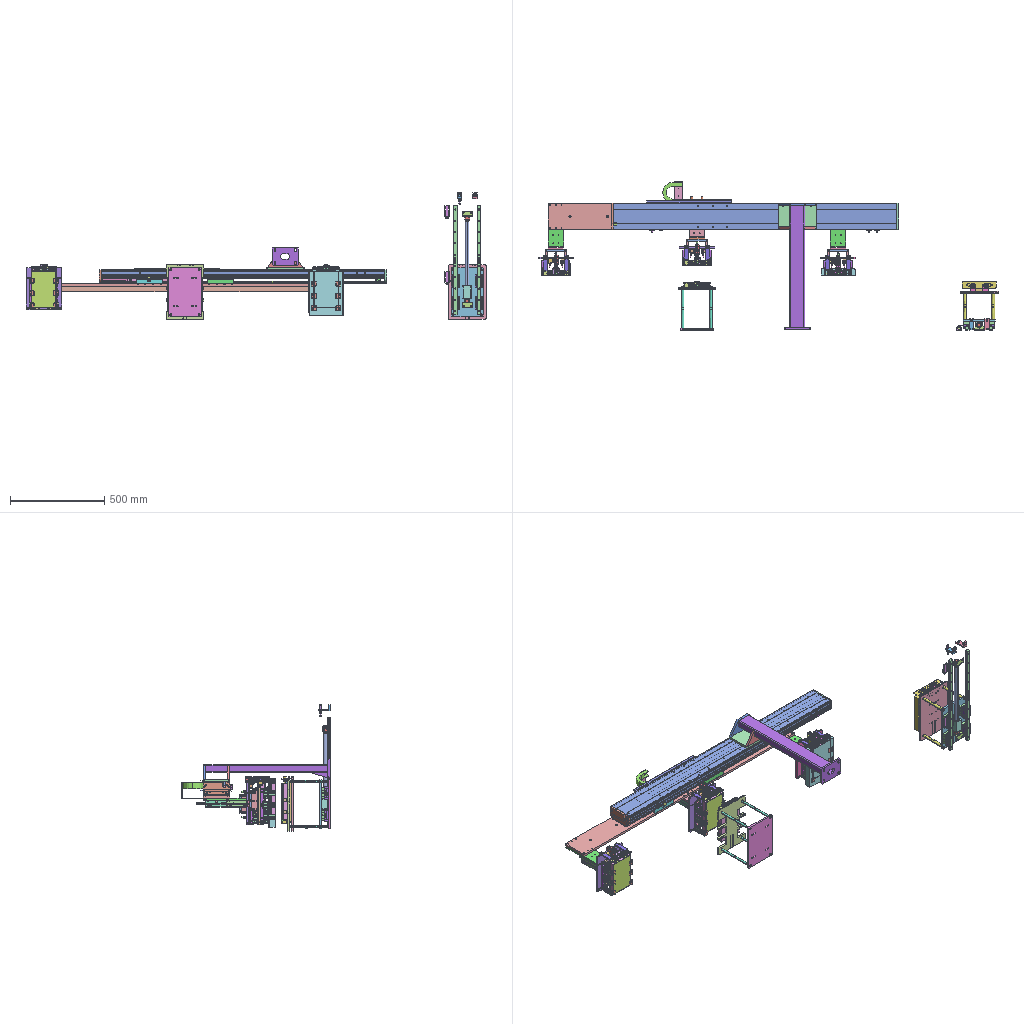Assembly | STEP file | 111 different items | 296 placed | box 2445 x 787 x 674 mm
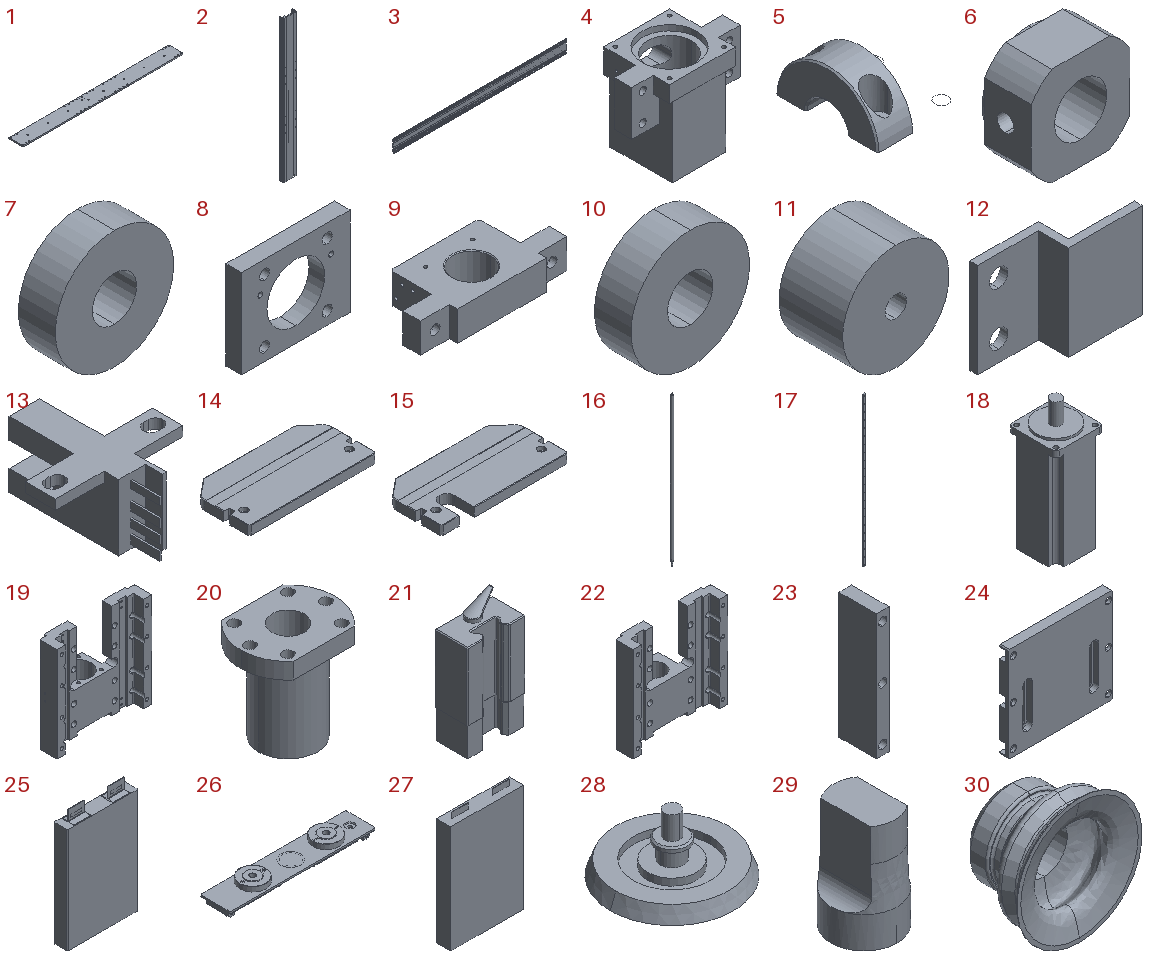Parts list (item | name | quantity | parent item | size | volume):
1 | 0-19-01 Sliding plate | x1 | in 33 | 1583 x 140 x 12 mm | 2630174 mm3
2 | SM140A-20-1140D-140A-600 Base SF600 | x1 | in SM140A-20-1140D-E | 140 x 48 x 1508 mm | 3406004 mm3
3 | SM140A-20-1140D-140A-600 Upper cover SF600 | x1 | in SM140A-20-1140D-E | 1524 x 10 x 112 mm | 391118 mm3
4 | SM140A-20-1140D-140A-600 Front bearing seat | x1 | in SM140A-20-1140D-E | 99 x 60 x 82 mm | 158063 mm3
5 | SM140A-20-1140D-140A-600 Coupling | x1 | in SM140A-20-1140D-E | - | -
6 | SM140A-20-1140D-140A-600 Lock nut | x1 | in SM140A-20-1140D-E | 19 x 10 x 19 mm | 2441 mm3
7 | SM140A-20-1140D-140A-600 Front bearing | x2 | in SM140A-20-1140D-E | 32 x 10 x 32 mm | 6912 mm3
8 | SM140A-20-1140D-140A-600 Pressure plate | x1 | in SM140A-20-1140D-E | 49 x 7 x 40 mm | 8955 mm3
9 | SM140A-20-1140D-140A-600 Rear bearing seat | x1 | in SM140A-20-1140D-E | 99 x 45.5 x 20 mm | 51169 mm3
10 | SM140A-20-1140D-140A-600 Rear end bearing | x1 | in SM140A-20-1140D-E | 26 x 8 x 26 mm | 3619 mm3
11 | SM140A-20-1140D-140A-600 Buffer pad | x4 | in SM140A-20-1140D-E | 15 x 9 x 15 mm | 1428 mm3
12 | SM140A-20-1140D-140A-600 External sensor plate | x1 | in SM140A-20-1140D-E | 25.5 x 7.25 x 18 mm | 814.887 mm3
13 | SM140A-20-1140D-140A-600ABSR | x3 | in SM140A-20-1140D-E | 26 x 28.4 x 13.5 mm | 1855 mm3
14 | SM140A-20-1140D-140A-600 Rear end plate | x1 | in SM140A-20-1140D-E | 140 x 70.5 x 10 mm | 88188 mm3
15 | SM140A-20-1140D-140A-600 Front end plate | x1 | in SM140A-20-1140D-E | 140 x 70.5 x 10 mm | 83515 mm3
16 | SM140A-20-1140D-140A-60016 Lead screw | x1 | in SM140A-20-1140D-E | 20 x 20 x 1305 mm | 397382 mm3
17 | SM140A-20-1140D-140A-600 Guide rail 600 | x2 | in SM140A-20-1140D-E | 15 x 12.5 x 1284 mm | 233266 mm3
18 | SM140A-20-1140D-Delta motor 400W | x1 | in SM140A-20-1140D-E | 60 x 60 x 160.7 mm | 433057 mm3
19 | SM140A-20-1140D-Slide plate 140-1000-2 | x1 | in SM140A-20-1140D-E | 140 x 58 x 140 mm | 247713 mm3
20 | SM140A-20-1140D-Slide plate 140-1000 -1000-2 | x1 | in SM140A-20-1140D-E | 58 x 44 x 60 mm | 52790 mm3
21 | SM140A-20-1140D-SM140F-140w-700EGH15SA | x2 | in SM140A-20-1140D-E | 34 x 19.5 x 66.139 mm | 30467 mm3
22 | SM140A-20-1140D-Side slide plate | x1 | in SM140A-20-1140D-E | 140 x 58 x 140 mm | 271598 mm3
23 | 0-09-15 Support plate | x6 | in 0-19-2 Gripper assembly 1, 0-19-1 Gripper assembly, 0-19-2 Gripper assembly 2 | 10 x 30 x 100 mm | 26921 mm3
24 | 0-19-15 Cylinder connecting plate | x3 | in 0-19-2 Gripper assembly 1, 0-19-1 Gripper assembly, 0-19-2 Gripper assembly 2 | 110 x 10 x 100 mm | 97973 mm3
25 | Inspection cell weld | x3 | in 0-19-2 Gripper assembly 1, 0-19-1 Gripper assembly, 0-19-2 Gripper assembly 2 | 131 x 25.2 x 215 mm | 644339 mm3
26 | CAM72FI L14 Cover plate assembly | x4 | in CAM72 L14 | - | -
27 | Cell simplified | x4 | in CAM72 L14 | 131 x 25.5 x 205 mm | 651997 mm3
28 | Seal Pin Weld Part | x4 | in CAM72 L14 | 8 x 8 x 3.75 mm | 41.644 mm3
29 | Seal Pin Seal Part | x4 | in CAM72 L14 | 3.15 x 3.15 x 5.05 mm | 29.674 mm3
30 | PJG-30 | x6 | in Suction cup assembly | 29.715 x 18 x 29.715 mm | 4013 mm3
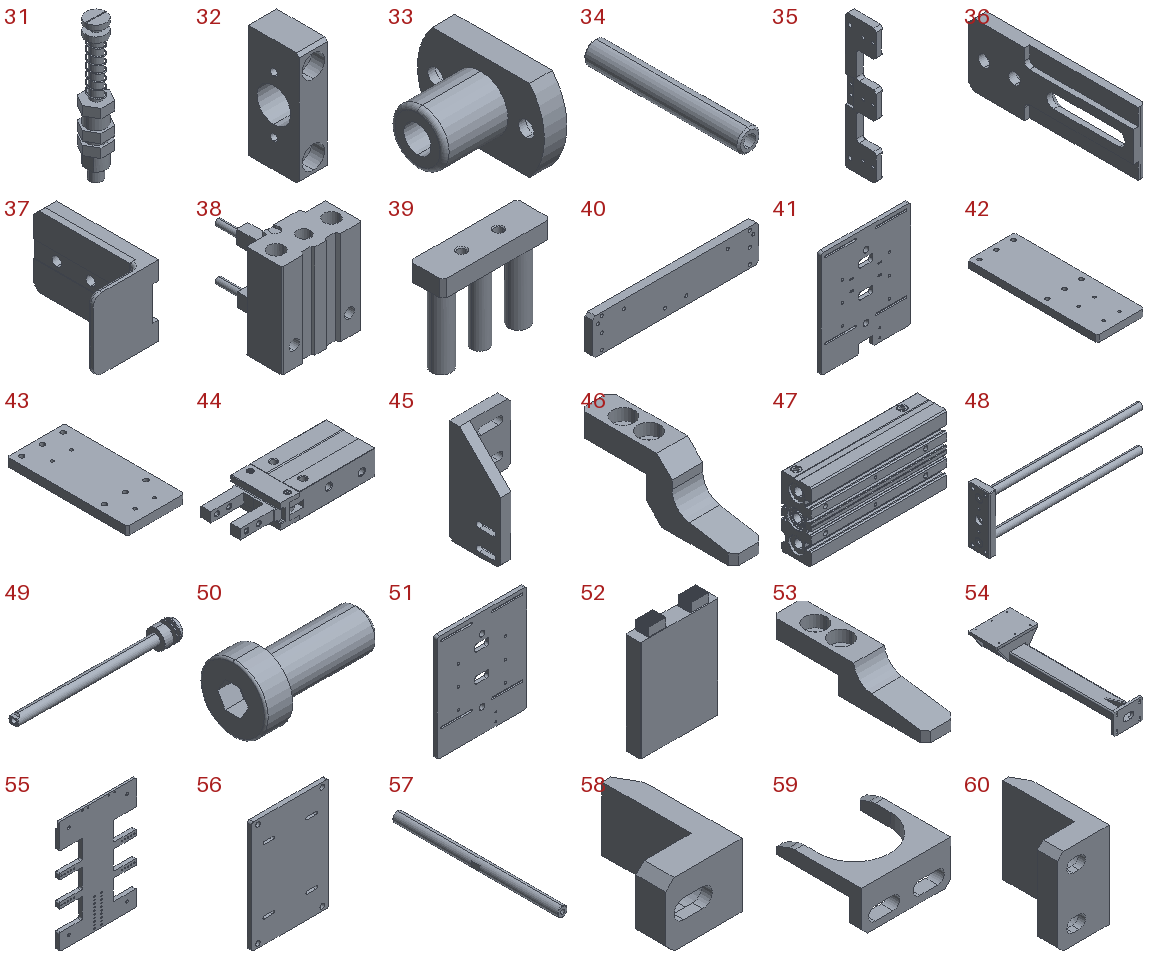31 | PJ90 | x6 | in Suction cup assembly | 15.011 x 13 x 77.2 mm | 5466 mm3
32 | 0-09-16 Linear bearing mount seat | x12 | in 0-10-3 Gripper assembly | 10 x 18 x 40 mm | 5072 mm3
33 | Flange linear bearing LMH6UUA | x12 | in 0-10-3 Gripper assembly | 19 x 28 x 18 mm | 3151 mm3
34 | 0-09-18 Guide shaft D6X50 | x12 | in 0-10-3 Gripper assembly | 6 x 42 x 6 mm | 1005 mm3
35 | 0-10-20 Support plate connecting plate | x6 | in 0-10-3 Gripper assembly | 8 x 38 x 163 mm | 31566 mm3
36 | 0-09-19 Support plate connecting plate | x18 | in 0-10-3 Gripper assembly | 5 x 65 x 25 mm | 5596 mm3
37 | 0-10-21 Cell support plate | x18 | in 0-10-3 Gripper assembly | 23 x 38 x 25 mm | 5641 mm3
38 | MGJ10-20-F8NL1 | x6 | in MGJ10-20-F8NL | 33 x 38.5 x 39 mm | 17194 mm3
39 | MGJ10-20-F8NL2 | x6 | in MGJ10-20-F8NL | 32 x 10 x 27 mm | 3209 mm3
40 | 0-10-28 Cylinder mounting plate | x6 | in 0-10-3 Gripper assembly | 180 x 8 x 39 mm | 55195 mm3
41 | 0-19-19 Mounting plate | x2 | in 0-19-2 Gripper assembly 1, 0-19-1 Gripper assembly | 190 x 8 x 225 mm | 312509 mm3
42 | 0-19-04 Lower cylinder mounting plate 1 | x2 | in 33 | 83 x 230 x 12 mm | 223254 mm3
43 | 0-19-05 Lower cylinder mounting plate 2 | x1 | in 33 | 83 x 175 x 12 mm | 168474 mm3
44 | HFZ6(CL)_HI | x2 | in HFZ6-CL-H-2_HI | 53 x 20 x 10 mm | 6778 mm3
45 | 0-19-02 Finger cylinder mounting plate | x2 | in 0-19-1 Gripper assembly, 0-19-2 Gripper assembly 2 | 30 x 30 x 60 mm | 12755 mm3
46 | 0-19-03 Finger | x2 | in 0-19-1 Gripper assembly | 6 x 30 x 12 mm | 793.591 mm3
47 | TC-L-20x125125_b_HI | x1 | in TC-L-20x125-S-G1-2 (0)_HI | 162 x 36 x 83 mm | 325855 mm3
48 | TC-L-20x125_125fp_HI | x1 | in TC-L-20x125-S-G1-2 (0)_HI | 229 x 30 x 81 mm | 57198 mm3
49 | TC-L-20x125_125r_HI | x1 | in TC-L-20x125-S-G1-2 (0)_HI | 164.5 x 19.9 x 19.9 mm | 15852 mm3
50 | TCL-TCM - 20_Screw_HI | x1 | in TC-L-20x125-S-G1-2 (0)_HI | 19 x 10 x 10 mm | 692.888 mm3
51 | 0-19-08 Connecting plate | x1 | in 0-19-2 Gripper assembly 2 | 190 x 8 x 225 mm | 317897 mm3
52 | Inspection cell max | x1 | in 0-19-2 Gripper assembly 2 | 180 x 35 x 255 mm | 1510927 mm3
53 | 0-19-07 Finger 2 | x2 | in 0-19-2 Gripper assembly 2 | 6 x 30 x 7 mm | 581.935 mm3
54 | 0-19-06 Mount seat_Default <Feature> | x1 | in 33 | 200 x 671.5 x 120 mm | 1373687 mm3
55 | 0-19-09 Discharge platform | x1 | in 0-19-4 Discharge platform | 200 x 10 x 290 mm | 370239 mm3
56 | 0-19-12 Mounting connecting plate | x1 | in 0-19-4 Discharge platform | 180 x 10 x 260 mm | 458114 mm3
57 | 0-19-13 Support rod | x4 | in 0-19-4 Discharge platform | 12 x 204 x 12 mm | 22364 mm3
58 | 0-05-02 Fixed side flange | x4 | in 0-19-4 Discharge platform | 18 x 28 x 15 mm | 2834 mm3
59 | 0-06-03 Cover plate locating block 1 | x2 | in 0-19-4 Discharge platform | 30 x 28.5 x 14 mm | 2389 mm3
60 | 0-05-07 Fixed side flange 3 | x1 | in 0-19-4 Discharge platform | 18 x 32 x 30 mm | 6534 mm3
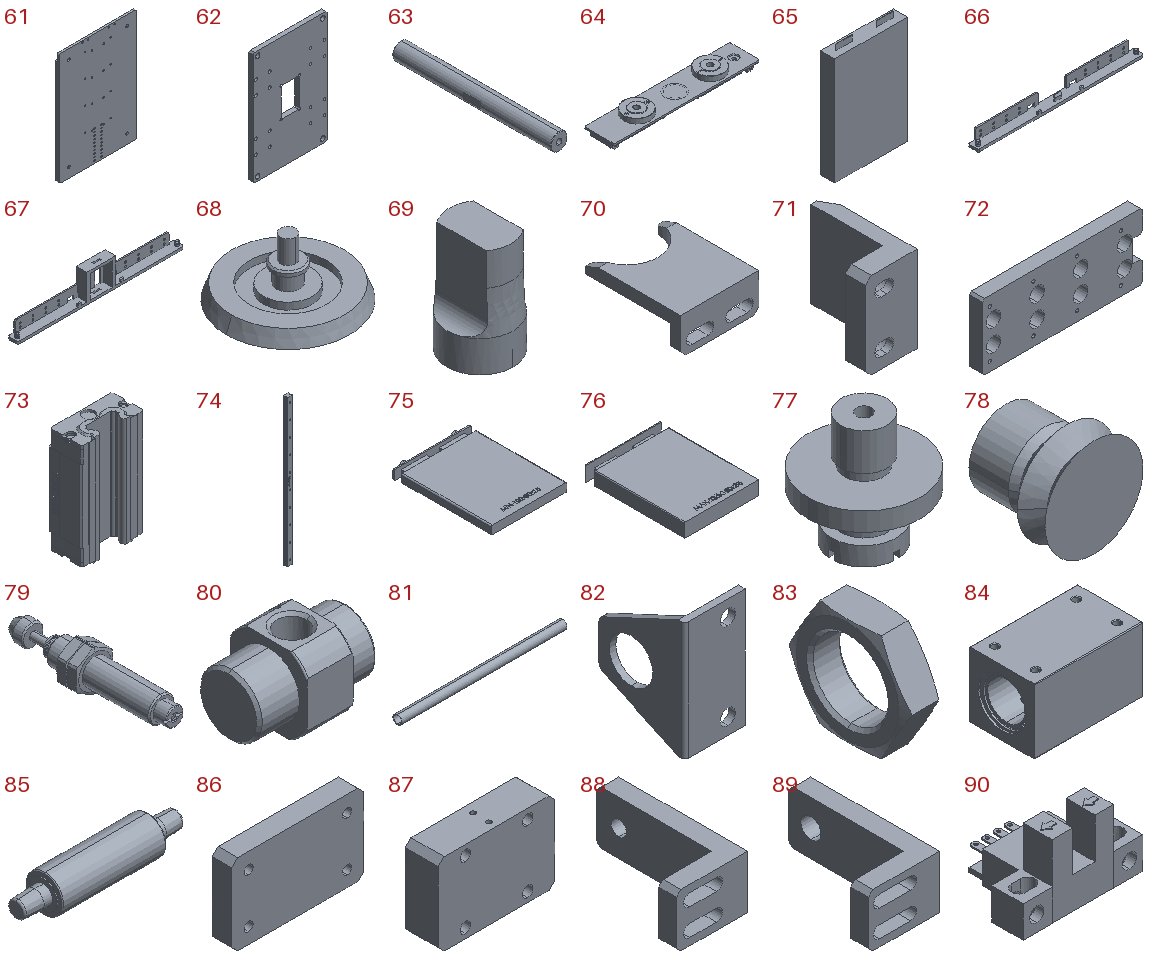61 | 0-19-09 Discharge platform 1 | x1 | in 0-19 Discharge platform 1 | 200 x 10 x 290 mm | 554142 mm3
62 | 0-19 Mounting plate 1 | x1 | in 0-19 Discharge platform 1 | 170 x 10 x 260 mm | 404759 mm3
63 | 0-19-13 Support rod 1 | x4 | in 0-19 Discharge platform 1 | 15 x 141 x 15 mm | 24242 mm3
64 | COMPANY_A-CAM72FI L14 Cover plate assembly | x2 | in COMPANY_A-CAM72 L14 | - | -
65 | COMPANY_A-Cell Simplified | x2 | in COMPANY_A-CAM72 L14 | 131 x 25.5 x 205 mm | 651997 mm3
66 | COMPANY_A-Bracket A | x2 | in COMPANY_A-CAM72 L14 | 129 x 8 x 10.5 mm | 2899 mm3
67 | COMPANY_A-Bracket B | x2 | in COMPANY_A-CAM72 L14 | 129 x 8 x 22 mm | 4052 mm3
68 | COMPANY_A-Seal Pin Weld Part | x2 | in COMPANY_A-CAM72 L14 | 8 x 8 x 3.75 mm | 41.644 mm3
69 | COMPANY_A-Seal Pin Seal Part | x2 | in COMPANY_A-CAM72 L14 | 3.15 x 3.15 x 5.05 mm | 29.674 mm3
70 | 0-019 Cover plate locating block (long) | x2 | in 0-19 Discharge platform 1 | 30 x 36.7 x 14 mm | 4576 mm3
71 | COMPANY_A-0-05 Fixed Block 1 | x1 | in 0-19 Discharge platform 1 | 18 x 32 x 30 mm | 6539 mm3
72 | 0-19 Battery pad plate | x1 | in 0-19 Discharge platform 1 | 220 x 18 x 91 mm | 303845 mm3
73 | EGH20CA Slider | x4 | in 0-19 Discharge platform 1 | 42 x 22.2 x 71.7 mm | 50391 mm3
74 | EGH20CA2R580Z0C,E=20MM | x2 | in 0-19 Discharge platform 1 | 20 x 15.5 x 580 mm | 158003 mm3
75 | MIN-Cell | x1 | in 0-19 Discharge platform 1 | 120 x 157 x 15 mm | 221771 mm3
76 | MAX-Cell | x1 | in 0-19 Discharge platform 1 | 180 x 245 x 35 mm | 1267148 mm3
77 | 0-19 Suction cup screw rod | x6 | in 0-19-001 Suction nozzle | 12 x 12 x 12 mm | 425.123 mm3
78 | JS2-20(0-19) | x6 | in 0-19-001 Suction nozzle | 20 x 18 x 20 mm | 3384 mm3
79 | ACA10 07-1(M10x1.0) | x1 | in 0-19 Discharge platform 1 | - | -
80 | RMS20X50_FCV | x2 | - | 38 x 25 x 25 mm | 12617 mm3
81 | - | x1 | - | 426 x 23 x 23 mm | 43129 mm3
82 | F_MF20LB_RMS_ | x2 | - | 28 x 40 x 55 mm | 7599 mm3
83 | RMS20X50_Nut | x2 | - | 8 x 30.022 x 26 mm | 2480 mm3
84 | RMS20X50_Body | x1 | - | 66 x 40 x 40 mm | 76860 mm3
85 | RMS20X50_Piston | x1 | - | 86 x 20 x 20 mm | 19878 mm3
86 | 0-19 Cylinder floating plate | x1 | in 0-19 Discharge platform 1 | 67 x 10 x 41 mm | 26049 mm3
87 | 0-19 Pad block | x4 | in 0-19 Discharge platform 1 | 60 x 17 x 42 mm | 40842 mm3
88 | 0-19 Buffer fixed 1 | x1 | in 0-19 Discharge platform 1 | 32 x 60 x 24 mm | 14337 mm3
89 | 0-19 Buffer fixed | x1 | in 0-19 Discharge platform 1 | 32 x 60 x 24 mm | 13943 mm3
90 | EE-SX671(OMRON) | x2 | in 0-19 Discharge platform 1 | 26.5 x 21 x 16.2 mm | 2322 mm3
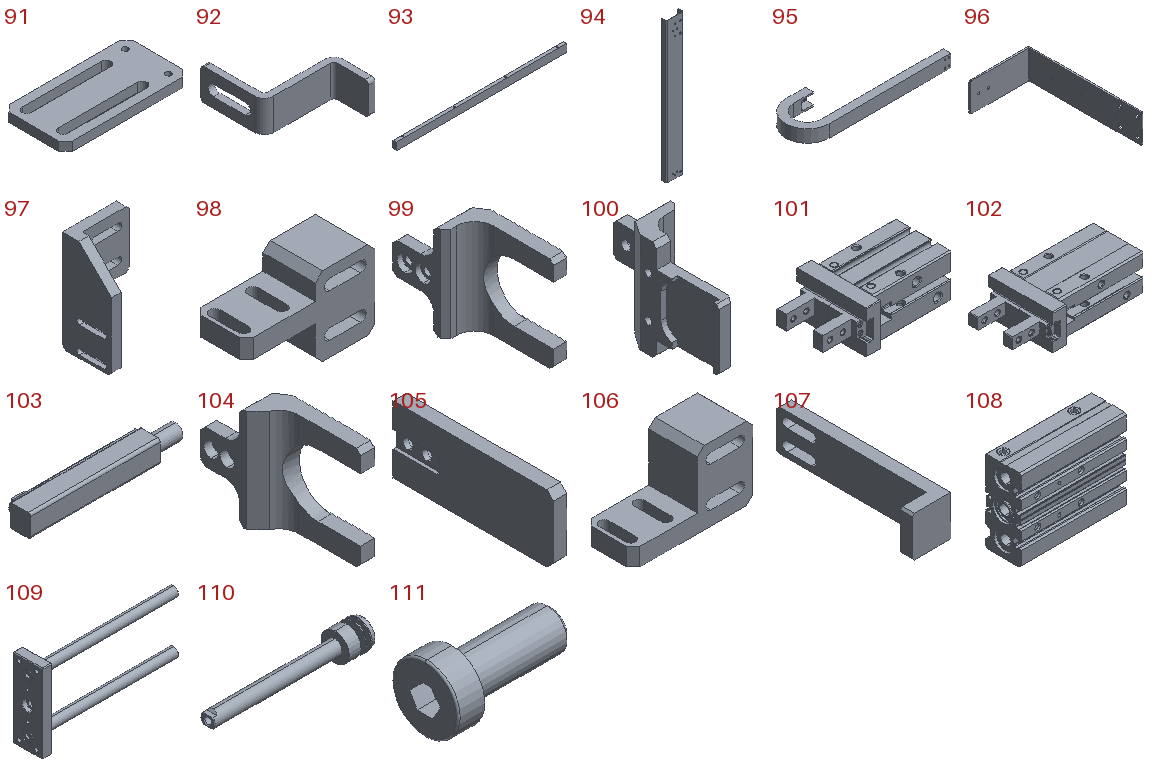91 | 0-22 Sensor seat | x2 | in 0-19 Discharge platform 1 | 55 x 28 x 4 mm | 4762 mm3
92 | 0-19-22 Sensor bracket | x1 | in 0-19 Discharge platform 1 | 24 x 31 x 10 mm | 934.705 mm3
93 | 0-19-14 Reinforcing rib | x2 | in 33 | 665 x 12 x 30 mm | 237897 mm3
94 | 0-19-21 Drag chain support plate | x1 | in 33 | 53 x 16.5 x 450 mm | 54218 mm3
95 | Drag chain MHPKS203-45-15-A3 | x1 | in 33 | 365 x 110 x 32 mm | 295090 mm3
96 | 0-19-20 Drag chain bracket | x1 | in 33 | 84 x 160 x 40 mm | 19040 mm3
97 | 0-19 Finger cylinder fixed plate 1 (original) | x1 | in 33 | 35 x 30 x 62 mm | 14067 mm3
98 | 0-19 Finger cylinder fixed plate | x1 | in 33 | 54 x 22 x 33 mm | 18394 mm3
99 | 0-19 Finger 2 | x2 | in 0-19 Pneumatic gripper | 16 x 50 x 36 mm | 5757 mm3
100 | 0-19 Finger 1 | x2 | in 0-19 Pneumatic gripper | 16 x 50 x 36 mm | 5853 mm3
101 | HFZ16(CL)_HI | x2 | in HFZ16-CL-H-2_HI | 67.3 x 38 x 23.6 mm | 30935 mm3
102 | HFZ10_CL_ | x1 | in HFZ10_CL_G1_2_HFZ10-CL-G1-2 | 57 x 29 x 16.4 mm | 14372 mm3
103 | CS1_G | x2 | in HFZ10_CL_G1_2_HFZ10-CL-G1-2 | 30.5 x 5.5 x 4.4 mm | 552.742 mm3
104 | 0-19 Finger 2 (original) | x1 | in 0-19 Pneumatic gripper (small) | 13 x 48 x 36 mm | 5429 mm3
105 | 0-19 Finger (retainer) | x1 | in 0-19 Pneumatic gripper (small) | 4 x 48 x 20 mm | 3676 mm3
106 | 0-19 Finger cylinder fixed plate 12 | x1 | in 33 | 54 x 22 x 33 mm | 18493 mm3
107 | 0-19-08 Cover plate block | x6 | in 33 | 19 x 80 x 20 mm | 10309 mm3
108 | TC_L_20x7070_b | x2 | - | 107 x 36 x 83 mm | 222327 mm3
109 | TC_L_20x70_70fp | x2 | - | 150 x 30 x 81 mm | 44789 mm3
110 | TC_L_20x70_70r | x2 | - | 109.5 x 19.9 x 19.9 mm | 11532 mm3
111 | - | x2 | - | 19 x 10 x 10 mm | 692.888 mm3
Placements (level | parent | child | x y z in mm | rotation matrix by rows), first 250 of 344 lines:
1 | 33 | 0-19-01 Sliding plate | 113.219 -17.373 0.0 | 1 0 0 0 1 0 0 0 1
1 | 33 | SM140A-20-1140D-E | -107.781 -10.138 66.544 | 0 0 1 -1 0 0 0 -1 0
2 | SM140A-20-1140D-E | SM140A-20-1140D-140A-600 Base SF600 | 7.235 -15.456 -225.0 | 1 0 0 0 1 0 0 0 1
2 | SM140A-20-1140D-E | SM140A-20-1140D-140A-600 Upper cover SF600 | 7.235 57.544 1291.0 | 0 0 1 0 1 0 -1 0 -0
2 | SM140A-20-1140D-E | SM140A-20-1140D-140A-600 Front bearing seat | 7.235 -7.456 -46.0 | -1 0 0 0 1 0 0 0 -1
2 | SM140A-20-1140D-E | SM140A-20-1140D-140A-600 Coupling | 5.454 21.554 -57.77 | 0 -0.8173 -0.5762 0 0.5762 -0.8173 1 0 0
2 | SM140A-20-1140D-E | SM140A-20-1140D-140A-600 Lock nut | 7.235 22.544 -35.0 | -0.9815 0 -0.1913 -0.1913 0 0.9815 0 1 0
2 | SM140A-20-1140D-E | SM140A-20-1140D-140A-600 Front bearing | 7.235 22.544 -5.0 | -0.1263 0 -0.992 0.992 0 -0.1263 0 -1 0
2 | SM140A-20-1140D-E | SM140A-20-1140D-140A-600 Front bearing | 7.235 22.544 -15.0 | 0.4269 0 0.9043 -0.9043 0 0.4269 0 -1 -0
2 | SM140A-20-1140D-E | SM140A-20-1140D-140A-600 Pressure plate | 7.235 42.544 -5.0 | -1 0 0 0 0 1 0 1 0
2 | SM140A-20-1140D-E | SM140A-20-1140D-140A-600 Rear bearing seat | 7.235 2.044 1261.0 | -1 0 0 0 1 0 0 0 -1
2 | SM140A-20-1140D-E | SM140A-20-1140D-140A-600 Rear end bearing | 7.235 22.544 1243.0 | 1 0 0 0 0 -1 0 1 0
2 | SM140A-20-1140D-E | SM140A-20-1140D-140A-600 Buffer pad | -8.765 29.544 2.0 | -0.7173 0 -0.6968 -0.6968 0 0.7173 0 1 -0
2 | SM140A-20-1140D-E | SM140A-20-1140D-140A-600 Buffer pad | 23.235 29.544 2.0 | -0.6066 0 0.795 0.795 0 0.6066 0 1 0
2 | SM140A-20-1140D-E | SM140A-20-1140D-140A-600 Buffer pad | 23.235 37.544 1241.0 | 0.8743 0 -0.4855 0.4855 0 0.8743 0 -1 0
2 | SM140A-20-1140D-E | SM140A-20-1140D-140A-600 Buffer pad | -8.765 37.544 1241.0 | 0.3714 0 0.9285 -0.9285 0 0.3714 0 -1 -0
2 | SM140A-20-1140D-E | SM140A-20-1140D-140A-600 External sensor plate | 77.235 47.044 40.0 | 0 -1 0 -1 0 0 0 0 -1
2 | SM140A-20-1140D-E | SM140A-20-1140D-140A-600ABSR | 79.235 11.794 1135.824 | 0 0 -1 0 1 0 1 0 -0
2 | SM140A-20-1140D-E | SM140A-20-1140D-140A-600ABSR | 79.235 11.794 -18.031 | 0 0 -1 0 1 0 1 0 -0
2 | SM140A-20-1140D-E | SM140A-20-1140D-140A-600 Rear end plate | 7.235 -12.956 1283.0 | 1 0 0 0 1 0 0 0 1
2 | SM140A-20-1140D-E | SM140A-20-1140D-140A-600 Front end plate | 7.235 -12.956 -225.0 | -1 0 0 0 1 0 0 0 -1
2 | SM140A-20-1140D-E | SM140A-20-1140D-140A-60016 Lead screw | 7.235 22.544 -50.0 | -0.602 0.7985 0 -0.7985 -0.602 0 0 0 1
2 | SM140A-20-1140D-E | SM140A-20-1140D-140A-600 Guide rail 600 | -35.765 13.794 -45.0 | 1 0 0 0 1 0 0 0 1
2 | SM140A-20-1140D-E | SM140A-20-1140D-140A-600 Guide rail 600 | 50.235 13.794 -45.0 | 1 0 0 0 1 0 0 0 1
2 | SM140A-20-1140D-E | SM140A-20-1140D-Delta motor 400W | 7.235 22.544 -217.7 | 1 0 0 0 1 0 0 0 1
2 | SM140A-20-1140D-E | SM140A-20-1140D-140A-600ABSR | 79.235 11.794 1175.87 | 0 0 -1 0 1 0 1 0 -0
2 | SM140A-20-1140D-E | SM140A-20-1140D-Slide plate 140-1000-2 | 7.235 2.544 101.0 | 1 0 0 0 -1 0 0 0 -1
2 | SM140A-20-1140D-E | SM140A-20-1140D-Slide plate 140-1000 -1000-2 | 7.235 22.544 91.0 | 1 0 0 0 -1 0 0 0 -1
2 | SM140A-20-1140D-E | SM140A-20-1140D-SM140F-140w-700EGH15SA | -52.765 12.044 59.3 | 1 0 0 0 1 0 0 0 1
2 | SM140A-20-1140D-E | SM140A-20-1140D-SM140F-140w-700EGH15SA | -18.765 12.044 12.7 | -1 0 0 0 1 0 0 0 -1
2 | SM140A-20-1140D-E | SM140A-20-1140D-Side slide plate | 7.235 2.544 481.0 | 1 0 0 0 -1 0 0 0 -1
1 | 33 | 0-19-2 Gripper assembly 1 | -678.281 -60.373 -54.0 | -1 0 0 0 1 0 0 0 -1
2 | 0-19-2 Gripper assembly 1 | 0-09-15 Support plate | -91.5 -158.0 -33.25 | 1 0 0 0 1 0 0 0 1
2 | 0-19-2 Gripper assembly 1 | 0-19-15 Cylinder connecting plate | -41.5 -138.0 -33.25 | -1 0 0 0 1 0 0 0 -1
2 | 0-19-2 Gripper assembly 1 | 0-09-15 Support plate | 8.5 -158.0 -33.25 | 1 0 0 0 1 0 0 0 1
2 | 0-19-2 Gripper assembly 1 | Inspection cell weld | -41.5 -258.4 -30.5 | -1 0 0 0 1 0 0 0 -1
2 | 0-19-2 Gripper assembly 1 | CAM72 L14 | -63.881 -268.793 -141.4 | -1 0 0 0 1 0 0 0 -1
3 | CAM72 L14 | CAM72FI L14 Cover plate assembly | -21.205 10.627 3.35 | 1 0 0 0 1 0 0 0 1
3 | CAM72 L14 | Cell simplified | -22.381 10.543 -208.4 | 1 0 0 0 1 0 0 0 1
3 | CAM72 L14 | Seal Pin Weld Part | 35.019 10.543 5.3 | -0.9237 -0.383 0 -0.383 0.9237 0 0 0 -1
3 | CAM72 L14 | Seal Pin Seal Part | 35.019 10.543 4.35 | -0.9237 -0.383 0 -0.383 0.9237 0 0 0 -1
2 | 0-19-2 Gripper assembly 1 | Suction cup assembly | -31.229 -227.854 2.683 | 0.1038 0 -0.9946 0 1 0 0.9946 0 0.1038
3 | Suction cup assembly | PJG-30 | -98.967 -9.146 -0.0 | 1 0 0 0 1 0 0 0 1
3 | Suction cup assembly | PJ90 | -98.967 41.354 -0.0 | 1 0 0 0 0 -1 0 1 0
2 | 0-19-2 Gripper assembly 1 | Suction cup assembly | -31.229 -227.854 137.683 | 0.1038 0 -0.9946 0 1 0 0.9946 0 0.1038
3 | Suction cup assembly | PJG-30 | -98.967 -9.146 -0.0 | 1 0 0 0 1 0 0 0 1
3 | Suction cup assembly | PJ90 | -98.967 41.354 -0.0 | 1 0 0 0 0 -1 0 1 0
2 | 0-19-2 Gripper assembly 1 | 0-10-3 Gripper assembly | 14.75 -198.0 -80.75 | 1 0 0 0 1 0 0 0 1
3 | 0-10-3 Gripper assembly | 0-09-16 Linear bearing mount seat | -1.25 0.0 -0.0 | 1 0 0 0 1 0 0 0 1
3 | 0-10-3 Gripper assembly | 0-09-16 Linear bearing mount seat | -1.25 -0.0 140.0 | -1 0 0 0 1 0 0 0 -1
3 | 0-10-3 Gripper assembly | Flange linear bearing LMH6UUA | -10.25 -0.0 140.0 | 1 0 0 0 0 1 0 -1 -0
3 | 0-10-3 Gripper assembly | Flange linear bearing LMH6UUA | -10.25 0.0 -0.0 | 1 0 0 0 0 1 0 -1 0
3 | 0-10-3 Gripper assembly | 0-09-18 Guide shaft D6X50 | -31.25 0.0 -0.0 | 0 1 0 -0.6761 0 -0.7368 -0.7368 0 0.6761
3 | 0-10-3 Gripper assembly | 0-09-18 Guide shaft D6X50 | -31.25 -0.0 140.0 | 0 1 0 -0.6231 0 -0.7821 -0.7821 0 0.6231
3 | 0-10-3 Gripper assembly | 0-10-20 Support plate connecting plate | 14.75 -13.0 70.0 | 1 0 0 0 1 0 0 0 1
3 | 0-10-3 Gripper assembly | 0-09-19 Support plate connecting plate | 16.75 -42.5 135.0 | 1 0 0 0 1 0 0 0 1
3 | 0-10-3 Gripper assembly | 0-10-21 Cell support plate | 7.25 -56.0 135.0 | 1 0 0 0 1 0 0 0 1
3 | 0-10-3 Gripper assembly | 0-09-19 Support plate connecting plate | 16.75 -42.5 70.0 | 1 0 0 0 1 0 0 0 1
3 | 0-10-3 Gripper assembly | 0-09-19 Support plate connecting plate | 16.75 -42.5 5.0 | 1 0 0 0 1 0 0 0 1
3 | 0-10-3 Gripper assembly | 0-10-21 Cell support plate | 7.25 -56.0 70.0 | 1 0 0 0 1 0 0 0 1
3 | 0-10-3 Gripper assembly | 0-10-21 Cell support plate | 7.25 -56.0 5.0 | 1 0 0 0 1 0 0 0 1
3 | 0-10-3 Gripper assembly | MGJ10-20-F8NL | 7.75 1.5 70.0 | 0 0 1 0 -1 0 1 0 0
4 | MGJ10-20-F8NL | MGJ10-20-F8NL1 | -0.0 -0.0 -0.0 | 1 0 0 0 1 0 0 0 1
4 | MGJ10-20-F8NL | MGJ10-20-F8NL2 | -0.0 -0.0 -0.0 | 1 0 0 0 1 0 0 0 1
3 | 0-10-3 Gripper assembly | 0-10-28 Cylinder mounting plate | 7.75 9.0 70.0 | 0 0 1 0 1 0 -1 0 -0
2 | 0-19-2 Gripper assembly 1 | 0-10-3 Gripper assembly | -97.75 -198.0 59.25 | -1 0 0 0 1 0 0 0 -1
3 | 0-10-3 Gripper assembly | 0-09-16 Linear bearing mount seat | -1.25 0.0 -0.0 | 1 0 0 0 1 0 0 0 1
3 | 0-10-3 Gripper assembly | 0-09-16 Linear bearing mount seat | -1.25 -0.0 140.0 | -1 0 0 0 1 0 0 0 -1
3 | 0-10-3 Gripper assembly | Flange linear bearing LMH6UUA | -10.25 -0.0 140.0 | 1 0 0 0 0 1 0 -1 -0
3 | 0-10-3 Gripper assembly | Flange linear bearing LMH6UUA | -10.25 0.0 -0.0 | 1 0 0 0 0 1 0 -1 0
3 | 0-10-3 Gripper assembly | 0-09-18 Guide shaft D6X50 | -31.25 0.0 -0.0 | 0 1 0 -0.6761 0 -0.7368 -0.7368 0 0.6761
3 | 0-10-3 Gripper assembly | 0-09-18 Guide shaft D6X50 | -31.25 -0.0 140.0 | 0 1 0 -0.6231 0 -0.7821 -0.7821 0 0.6231
3 | 0-10-3 Gripper assembly | 0-10-20 Support plate connecting plate | 14.75 -13.0 70.0 | 1 0 0 0 1 0 0 0 1
3 | 0-10-3 Gripper assembly | 0-09-19 Support plate connecting plate | 16.75 -42.5 135.0 | 1 0 0 0 1 0 0 0 1
3 | 0-10-3 Gripper assembly | 0-10-21 Cell support plate | 7.25 -56.0 135.0 | 1 0 0 0 1 0 0 0 1
3 | 0-10-3 Gripper assembly | 0-09-19 Support plate connecting plate | 16.75 -42.5 70.0 | 1 0 0 0 1 0 0 0 1
3 | 0-10-3 Gripper assembly | 0-09-19 Support plate connecting plate | 16.75 -42.5 5.0 | 1 0 0 0 1 0 0 0 1
3 | 0-10-3 Gripper assembly | 0-10-21 Cell support plate | 7.25 -56.0 70.0 | 1 0 0 0 1 0 0 0 1
3 | 0-10-3 Gripper assembly | 0-10-21 Cell support plate | 7.25 -56.0 5.0 | 1 0 0 0 1 0 0 0 1
3 | 0-10-3 Gripper assembly | MGJ10-20-F8NL | 7.75 1.5 70.0 | 0 0 1 0 -1 0 1 0 0
4 | MGJ10-20-F8NL | MGJ10-20-F8NL1 | -0.0 -0.0 -0.0 | 1 0 0 0 1 0 0 0 1
4 | MGJ10-20-F8NL | MGJ10-20-F8NL2 | -0.0 -0.0 -0.0 | 1 0 0 0 1 0 0 0 1
3 | 0-10-3 Gripper assembly | 0-10-28 Cylinder mounting plate | 7.75 9.0 70.0 | 0 0 1 0 1 0 -1 0 -0
2 | 0-19-2 Gripper assembly 1 | 0-19-19 Mounting plate | -41.5 -177.0 -33.25 | 1 0 0 0 1 0 0 0 1
1 | 33 | 0-19-04 Lower cylinder mounting plate 1 | -636.781 -62.373 -12.0 | 1 0 0 0 1 0 0 0 1
1 | 33 | 0-19-04 Lower cylinder mounting plate 1 | 863.219 -62.373 -12.0 | 1 0 0 0 1 0 0 0 1
1 | 33 | 0-19-05 Lower cylinder mounting plate 2 | 113.219 -34.873 -12.0 | 1 0 0 0 1 0 0 0 1
1 | 33 | 0-19-1 Gripper assembly | 48.618 -29.957 -302.53 | -1 0 -0.003178 0 1 0 0.003178 0 -1
2 | 0-19-1 Gripper assembly | 0-19-19 Mounting plate | -63.754 -152.416 -266.734 | 1 0 -0.003178 0 1 0 0.003178 0 1
2 | 0-19-1 Gripper assembly | 0-09-15 Support plate | -113.754 -133.416 -266.893 | 1 0 -0.003178 0 1 0 0.003178 0 1
2 | 0-19-1 Gripper assembly | 0-19-15 Cylinder connecting plate | -63.754 -113.416 -266.734 | 1 0 -0.003178 0 1 0 0.003178 0 1
2 | 0-19-1 Gripper assembly | 0-09-15 Support plate | -13.754 -133.416 -266.575 | 1 0 -0.003178 0 1 0 0.003178 0 1
2 | 0-19-1 Gripper assembly | Inspection cell weld | -63.714 -233.816 -279.234 | -1 0 0.003178 0 1 0 -0.003178 0 -1
2 | 0-19-1 Gripper assembly | CAM72 L14 | -85.743 -244.209 -390.204 | -1 0 0.003178 0 1 0 -0.003178 0 -1
3 | CAM72 L14 | CAM72FI L14 Cover plate assembly | -21.205 10.627 3.35 | 1 0 0 0 1 0 0 0 1
3 | CAM72 L14 | Cell simplified | -22.381 10.543 -208.4 | 1 0 0 0 1 0 0 0 1
3 | CAM72 L14 | Seal Pin Weld Part | 35.019 10.543 5.3 | -0.9237 -0.383 0 -0.383 0.9237 0 0 0 -1
3 | CAM72 L14 | Seal Pin Seal Part | 35.019 10.543 4.35 | -0.9237 -0.383 0 -0.383 0.9237 0 0 0 -1
2 | 0-19-1 Gripper assembly | HFZ6-CL-H-2_HI | -56.949 -156.416 -394.213 | 0 0.003178 -1 1 0 0 0 -1 -0.003178
3 | HFZ6-CL-H-2_HI | HFZ6(CL)_HI | 0.0 0.0 -0.0 | 1 0 0 0 1 0 0 0 1
2 | 0-19-1 Gripper assembly | 0-19-02 Finger cylinder mounting plate | -37.013 -171.416 -374.149 | 1 0 -0.003178 0 1 0 0.003178 0 1
2 | 0-19-1 Gripper assembly | 0-19-03 Finger | -56.97 -211.416 -387.703 | 1 0 -0.003178 0 1 0 0.003178 0 1
2 | 0-19-1 Gripper assembly | 0-19-03 Finger | -56.928 -211.416 -400.723 | -1 0 0.003178 0 1 0 -0.003178 0 -1
2 | 0-19-1 Gripper assembly | Suction cup assembly | 35.411 -203.27 -329.233 | 1 0 0 0 1 0 0 0 1
3 | Suction cup assembly | PJG-30 | -98.967 -9.146 -0.0 | 1 0 0 0 1 0 0 0 1
3 | Suction cup assembly | PJ90 | -98.967 41.354 -0.0 | 1 0 0 0 0 -1 0 1 0
2 | 0-19-1 Gripper assembly | Suction cup assembly | 34.983 -203.27 -194.234 | 1 0 0 0 1 0 0 0 1
3 | Suction cup assembly | PJG-30 | -98.967 -9.146 -0.0 | 1 0 0 0 1 0 0 0 1
3 | Suction cup assembly | PJ90 | -98.967 41.354 -0.0 | 1 0 0 0 0 -1 0 1 0
2 | 0-19-1 Gripper assembly | 0-10-3 Gripper assembly | -7.354 -173.416 -314.055 | 1 0 -0.003178 0 1 0 0.003178 0 1
3 | 0-10-3 Gripper assembly | 0-09-16 Linear bearing mount seat | -1.25 0.0 -0.0 | 1 0 0 0 1 0 0 0 1
3 | 0-10-3 Gripper assembly | 0-09-16 Linear bearing mount seat | -1.25 -0.0 140.0 | -1 0 0 0 1 0 0 0 -1
3 | 0-10-3 Gripper assembly | Flange linear bearing LMH6UUA | -10.25 -0.0 140.0 | 1 0 0 0 0 1 0 -1 -0
3 | 0-10-3 Gripper assembly | Flange linear bearing LMH6UUA | -10.25 0.0 -0.0 | 1 0 0 0 0 1 0 -1 0
3 | 0-10-3 Gripper assembly | 0-09-18 Guide shaft D6X50 | -31.25 0.0 -0.0 | 0 1 0 -0.6761 0 -0.7368 -0.7368 0 0.6761
3 | 0-10-3 Gripper assembly | 0-09-18 Guide shaft D6X50 | -31.25 -0.0 140.0 | 0 1 0 -0.6231 0 -0.7821 -0.7821 0 0.6231
3 | 0-10-3 Gripper assembly | 0-10-20 Support plate connecting plate | 14.75 -13.0 70.0 | 1 0 0 0 1 0 0 0 1
3 | 0-10-3 Gripper assembly | 0-09-19 Support plate connecting plate | 16.75 -42.5 135.0 | 1 0 0 0 1 0 0 0 1
3 | 0-10-3 Gripper assembly | 0-10-21 Cell support plate | 7.25 -56.0 135.0 | 1 0 0 0 1 0 0 0 1
3 | 0-10-3 Gripper assembly | 0-09-19 Support plate connecting plate | 16.75 -42.5 70.0 | 1 0 0 0 1 0 0 0 1
3 | 0-10-3 Gripper assembly | 0-09-19 Support plate connecting plate | 16.75 -42.5 5.0 | 1 0 0 0 1 0 0 0 1
3 | 0-10-3 Gripper assembly | 0-10-21 Cell support plate | 7.25 -56.0 70.0 | 1 0 0 0 1 0 0 0 1
3 | 0-10-3 Gripper assembly | 0-10-21 Cell support plate | 7.25 -56.0 5.0 | 1 0 0 0 1 0 0 0 1
3 | 0-10-3 Gripper assembly | MGJ10-20-F8NL | 7.75 1.5 70.0 | 0 0 1 0 -1 0 1 0 0
4 | MGJ10-20-F8NL | MGJ10-20-F8NL1 | -0.0 -0.0 -0.0 | 1 0 0 0 1 0 0 0 1
4 | MGJ10-20-F8NL | MGJ10-20-F8NL2 | -0.0 -0.0 -0.0 | 1 0 0 0 1 0 0 0 1
3 | 0-10-3 Gripper assembly | 0-10-28 Cylinder mounting plate | 7.75 9.0 70.0 | 0 0 1 0 1 0 -1 0 -0
2 | 0-19-1 Gripper assembly | 0-10-3 Gripper assembly | -120.298 -173.416 -174.413 | -1 0 0.003178 0 1 0 -0.003178 0 -1
3 | 0-10-3 Gripper assembly | 0-09-16 Linear bearing mount seat | -1.25 0.0 -0.0 | 1 0 0 0 1 0 0 0 1
3 | 0-10-3 Gripper assembly | 0-09-16 Linear bearing mount seat | -1.25 -0.0 140.0 | -1 0 0 0 1 0 0 0 -1
3 | 0-10-3 Gripper assembly | Flange linear bearing LMH6UUA | -10.25 -0.0 140.0 | 1 0 0 0 0 1 0 -1 -0
3 | 0-10-3 Gripper assembly | Flange linear bearing LMH6UUA | -10.25 0.0 -0.0 | 1 0 0 0 0 1 0 -1 0
3 | 0-10-3 Gripper assembly | 0-09-18 Guide shaft D6X50 | -31.25 0.0 -0.0 | 0 1 0 -0.6761 0 -0.7368 -0.7368 0 0.6761
3 | 0-10-3 Gripper assembly | 0-09-18 Guide shaft D6X50 | -31.25 -0.0 140.0 | 0 1 0 -0.6231 0 -0.7821 -0.7821 0 0.6231
3 | 0-10-3 Gripper assembly | 0-10-20 Support plate connecting plate | 14.75 -13.0 70.0 | 1 0 0 0 1 0 0 0 1
3 | 0-10-3 Gripper assembly | 0-09-19 Support plate connecting plate | 16.75 -42.5 135.0 | 1 0 0 0 1 0 0 0 1
3 | 0-10-3 Gripper assembly | 0-10-21 Cell support plate | 7.25 -56.0 135.0 | 1 0 0 0 1 0 0 0 1
3 | 0-10-3 Gripper assembly | 0-09-19 Support plate connecting plate | 16.75 -42.5 70.0 | 1 0 0 0 1 0 0 0 1
3 | 0-10-3 Gripper assembly | 0-09-19 Support plate connecting plate | 16.75 -42.5 5.0 | 1 0 0 0 1 0 0 0 1
3 | 0-10-3 Gripper assembly | 0-10-21 Cell support plate | 7.25 -56.0 70.0 | 1 0 0 0 1 0 0 0 1
3 | 0-10-3 Gripper assembly | 0-10-21 Cell support plate | 7.25 -56.0 5.0 | 1 0 0 0 1 0 0 0 1
3 | 0-10-3 Gripper assembly | MGJ10-20-F8NL | 7.75 1.5 70.0 | 0 0 1 0 -1 0 1 0 0
4 | MGJ10-20-F8NL | MGJ10-20-F8NL1 | -0.0 -0.0 -0.0 | 1 0 0 0 1 0 0 0 1
4 | MGJ10-20-F8NL | MGJ10-20-F8NL2 | -0.0 -0.0 -0.0 | 1 0 0 0 1 0 0 0 1
3 | 0-10-3 Gripper assembly | 0-10-28 Cylinder mounting plate | 7.75 9.0 70.0 | 0 0 1 0 1 0 -1 0 -0
1 | 33 | TC-L-20x125-S-G1-2 (0)_HI | 113.219 -122.373 -36.0 | 0 1 0 1 0 0 0 0 -1
2 | TC-L-20x125-S-G1-2 (0)_HI | TC-L-20x125125_b_HI | -0.0 -0.0 -0.0 | 1 0 0 0 0 -1 0 1 0
2 | TC-L-20x125-S-G1-2 (0)_HI | TC-L-20x125_125fp_HI | -16.0 -0.0 -0.0 | 1 0 0 0 0 -1 0 1 0
2 | TC-L-20x125-S-G1-2 (0)_HI | TC-L-20x125_125r_HI | -6.0 0.0 -0.0 | 1 0 0 0 1 0 0 0 1
2 | TC-L-20x125-S-G1-2 (0)_HI | TCL-TCM - 20_Screw_HI | -12.0 -0.0 -0.0 | 1 0 0 0 0 -1 0 1 0
1 | 33 | 0-19-2 Gripper assembly 2 | 798.618 -84.957 -302.53 | -1 0 -0.003178 0 1 0 0.003178 0 -1
2 | 0-19-2 Gripper assembly 2 | 0-19-08 Connecting plate | -63.754 -152.416 -266.734 | 1 0 -0.003178 0 1 0 0.003178 0 1
2 | 0-19-2 Gripper assembly 2 | 0-09-15 Support plate | -113.754 -133.416 -266.893 | 1 0 -0.003178 0 1 0 0.003178 0 1
2 | 0-19-2 Gripper assembly 2 | 0-19-15 Cylinder connecting plate | -63.754 -113.416 -266.734 | 1 0 -0.003178 0 1 0 0.003178 0 1
2 | 0-19-2 Gripper assembly 2 | 0-09-15 Support plate | -13.754 -133.416 -266.575 | 1 0 -0.003178 0 1 0 0.003178 0 1
2 | 0-19-2 Gripper assembly 2 | Inspection cell weld | -63.714 -233.816 -279.234 | -1 0 0.003178 0 1 0 -0.003178 0 -1
2 | 0-19-2 Gripper assembly 2 | Inspection cell max | -63.778 -228.916 -259.234 | -1 0 0.003178 0 1 0 -0.003178 0 -1
2 | 0-19-2 Gripper assembly 2 | CAM72 L14 | -85.743 -244.209 -390.204 | -1 0 0.003178 0 1 0 -0.003178 0 -1
3 | CAM72 L14 | CAM72FI L14 Cover plate assembly | -21.205 10.627 3.35 | 1 0 0 0 1 0 0 0 1
3 | CAM72 L14 | Cell simplified | -22.381 10.543 -208.4 | 1 0 0 0 1 0 0 0 1
3 | CAM72 L14 | Seal Pin Weld Part | 35.019 10.543 5.3 | -0.9237 -0.383 0 -0.383 0.9237 0 0 0 -1
3 | CAM72 L14 | Seal Pin Seal Part | 35.019 10.543 4.35 | -0.9237 -0.383 0 -0.383 0.9237 0 0 0 -1
2 | 0-19-2 Gripper assembly 2 | Suction cup assembly | 22.309 -203.27 -378.444 | 0.8676 0 0.4972 0 1 0 -0.4972 0 0.8676
3 | Suction cup assembly | PJG-30 | -98.967 -9.146 -0.0 | 1 0 0 0 1 0 0 0 1
3 | Suction cup assembly | PJ90 | -98.967 41.354 -0.0 | 1 0 0 0 0 -1 0 1 0
2 | 0-19-2 Gripper assembly 2 | Suction cup assembly | 21.88 -203.27 -243.445 | 0.8676 0 0.4972 0 1 0 -0.4972 0 0.8676
3 | Suction cup assembly | PJG-30 | -98.967 -9.146 -0.0 | 1 0 0 0 1 0 0 0 1
3 | Suction cup assembly | PJ90 | -98.967 41.354 -0.0 | 1 0 0 0 0 -1 0 1 0
2 | 0-19-2 Gripper assembly 2 | 0-10-3 Gripper assembly | -7.354 -173.416 -314.055 | 1 0 -0.003178 0 1 0 0.003178 0 1
3 | 0-10-3 Gripper assembly | 0-09-16 Linear bearing mount seat | -1.25 0.0 -0.0 | 1 0 0 0 1 0 0 0 1
3 | 0-10-3 Gripper assembly | 0-09-16 Linear bearing mount seat | -1.25 -0.0 140.0 | -1 0 0 0 1 0 0 0 -1
3 | 0-10-3 Gripper assembly | Flange linear bearing LMH6UUA | -10.25 -0.0 140.0 | 1 0 0 0 0 1 0 -1 -0
3 | 0-10-3 Gripper assembly | Flange linear bearing LMH6UUA | -10.25 0.0 -0.0 | 1 0 0 0 0 1 0 -1 0
3 | 0-10-3 Gripper assembly | 0-09-18 Guide shaft D6X50 | -31.25 0.0 -0.0 | 0 1 0 -0.6761 0 -0.7368 -0.7368 0 0.6761
3 | 0-10-3 Gripper assembly | 0-09-18 Guide shaft D6X50 | -31.25 -0.0 140.0 | 0 1 0 -0.6231 0 -0.7821 -0.7821 0 0.6231
3 | 0-10-3 Gripper assembly | 0-10-20 Support plate connecting plate | 14.75 -13.0 70.0 | 1 0 0 0 1 0 0 0 1
3 | 0-10-3 Gripper assembly | 0-09-19 Support plate connecting plate | 16.75 -42.5 135.0 | 1 0 0 0 1 0 0 0 1
3 | 0-10-3 Gripper assembly | 0-10-21 Cell support plate | 7.25 -56.0 135.0 | 1 0 0 0 1 0 0 0 1
3 | 0-10-3 Gripper assembly | 0-09-19 Support plate connecting plate | 16.75 -42.5 70.0 | 1 0 0 0 1 0 0 0 1
3 | 0-10-3 Gripper assembly | 0-09-19 Support plate connecting plate | 16.75 -42.5 5.0 | 1 0 0 0 1 0 0 0 1
3 | 0-10-3 Gripper assembly | 0-10-21 Cell support plate | 7.25 -56.0 70.0 | 1 0 0 0 1 0 0 0 1
3 | 0-10-3 Gripper assembly | 0-10-21 Cell support plate | 7.25 -56.0 5.0 | 1 0 0 0 1 0 0 0 1
3 | 0-10-3 Gripper assembly | MGJ10-20-F8NL | 7.75 1.5 70.0 | 0 0 1 0 -1 0 1 0 0
4 | MGJ10-20-F8NL | MGJ10-20-F8NL1 | -0.0 -0.0 -0.0 | 1 0 0 0 1 0 0 0 1
4 | MGJ10-20-F8NL | MGJ10-20-F8NL2 | -0.0 -0.0 -0.0 | 1 0 0 0 1 0 0 0 1
3 | 0-10-3 Gripper assembly | 0-10-28 Cylinder mounting plate | 7.75 9.0 70.0 | 0 0 1 0 1 0 -1 0 -0
2 | 0-19-2 Gripper assembly 2 | 0-10-3 Gripper assembly | -120.298 -173.416 -174.413 | -1 0 0.003178 0 1 0 -0.003178 0 -1
3 | 0-10-3 Gripper assembly | 0-09-16 Linear bearing mount seat | -1.25 0.0 -0.0 | 1 0 0 0 1 0 0 0 1
3 | 0-10-3 Gripper assembly | 0-09-16 Linear bearing mount seat | -1.25 -0.0 140.0 | -1 0 0 0 1 0 0 0 -1
3 | 0-10-3 Gripper assembly | Flange linear bearing LMH6UUA | -10.25 -0.0 140.0 | 1 0 0 0 0 1 0 -1 -0
3 | 0-10-3 Gripper assembly | Flange linear bearing LMH6UUA | -10.25 0.0 -0.0 | 1 0 0 0 0 1 0 -1 0
3 | 0-10-3 Gripper assembly | 0-09-18 Guide shaft D6X50 | -31.25 0.0 -0.0 | 0 1 0 -0.6761 0 -0.7368 -0.7368 0 0.6761
3 | 0-10-3 Gripper assembly | 0-09-18 Guide shaft D6X50 | -31.25 -0.0 140.0 | 0 1 0 -0.6231 0 -0.7821 -0.7821 0 0.6231
3 | 0-10-3 Gripper assembly | 0-10-20 Support plate connecting plate | 14.75 -13.0 70.0 | 1 0 0 0 1 0 0 0 1
3 | 0-10-3 Gripper assembly | 0-09-19 Support plate connecting plate | 16.75 -42.5 135.0 | 1 0 0 0 1 0 0 0 1
3 | 0-10-3 Gripper assembly | 0-10-21 Cell support plate | 7.25 -56.0 135.0 | 1 0 0 0 1 0 0 0 1
3 | 0-10-3 Gripper assembly | 0-09-19 Support plate connecting plate | 16.75 -42.5 70.0 | 1 0 0 0 1 0 0 0 1
3 | 0-10-3 Gripper assembly | 0-09-19 Support plate connecting plate | 16.75 -42.5 5.0 | 1 0 0 0 1 0 0 0 1
3 | 0-10-3 Gripper assembly | 0-10-21 Cell support plate | 7.25 -56.0 70.0 | 1 0 0 0 1 0 0 0 1
3 | 0-10-3 Gripper assembly | 0-10-21 Cell support plate | 7.25 -56.0 5.0 | 1 0 0 0 1 0 0 0 1
3 | 0-10-3 Gripper assembly | MGJ10-20-F8NL | 7.75 1.5 70.0 | 0 0 1 0 -1 0 1 0 0
4 | MGJ10-20-F8NL | MGJ10-20-F8NL1 | -0.0 -0.0 -0.0 | 1 0 0 0 1 0 0 0 1
4 | MGJ10-20-F8NL | MGJ10-20-F8NL2 | -0.0 -0.0 -0.0 | 1 0 0 0 1 0 0 0 1
3 | 0-10-3 Gripper assembly | 0-10-28 Cylinder mounting plate | 7.75 9.0 70.0 | 0 0 1 0 1 0 -1 0 -0
2 | 0-19-2 Gripper assembly 2 | HFZ6-CL-H-2_HI | -56.961 -156.416 -390.413 | 0 0.003178 -1 1 0 0 0 -1 -0.003178
3 | HFZ6-CL-H-2_HI | HFZ6(CL)_HI | 0.0 0.0 -0.0 | 1 0 0 0 1 0 0 0 1
2 | 0-19-2 Gripper assembly 2 | 0-19-02 Finger cylinder mounting plate | -37.025 -171.416 -370.349 | 1 0 -0.003178 0 1 0 0.003178 0 1
2 | 0-19-2 Gripper assembly 2 | 0-19-07 Finger 2 | -56.986 -211.416 -382.403 | 1 0 -0.003178 0 1 0 0.003178 0 1
2 | 0-19-2 Gripper assembly 2 | 0-19-07 Finger 2 | -56.936 -211.416 -398.423 | -1 0 0.003178 0 1 0 -0.003178 0 -1
1 | 33 | 0-19-06 Mount seat_Default <Feature> | 646.219 -285.123 151.5 | -1 0 0 0 1 0 0 0 -1
1 | 33 | 0-19-4 Discharge platform | 128.966 -386.493 -38.25 | 1 0 0 0 1 0 0 0 1
2 | 0-19-4 Discharge platform | 0-19-09 Discharge platform | -15.747 -15.38 -0.0 | 1 0 0 0 1 0 0 0 1
2 | 0-19-4 Discharge platform | 0-19-12 Mounting connecting plate | -15.747 -229.38 -0.0 | 1 0 0 0 1 0 0 0 1
2 | 0-19-4 Discharge platform | 0-19-13 Support rod | -90.747 -122.38 -120.0 | 0.01074 0 -0.9999 0 1 0 0.9999 0 0.01074
2 | 0-19-4 Discharge platform | 0-19-13 Support rod | -90.747 -122.38 120.0 | 0.01074 0 -0.9999 0 1 0 0.9999 0 0.01074
2 | 0-19-4 Discharge platform | 0-19-13 Support rod | 59.253 -122.38 -120.0 | -0.4429 0 -0.8966 0 1 0 0.8966 0 -0.4429
2 | 0-19-4 Discharge platform | 0-19-13 Support rod | 59.253 -122.38 120.0 | 0.01074 0 -0.9999 0 1 0 0.9999 0 0.01074
2 | 0-19-4 Discharge platform | CAM72 L14 | 6.634 -8.172 125.65 | 1 0 0 0 1 0 0 0 1
3 | CAM72 L14 | CAM72FI L14 Cover plate assembly | -21.205 10.627 3.35 | 1 0 0 0 1 0 0 0 1
3 | CAM72 L14 | Cell simplified | -22.381 10.543 -208.4 | 1 0 0 0 1 0 0 0 1
3 | CAM72 L14 | Seal Pin Weld Part | 35.019 10.543 5.3 | -0.9237 -0.383 0 -0.383 0.9237 0 0 0 -1
3 | CAM72 L14 | Seal Pin Seal Part | 35.019 10.543 4.35 | -0.9237 -0.383 0 -0.383 0.9237 0 0 0 -1
2 | 0-19-4 Discharge platform | 0-05-02 Fixed side flange | -79.997 -10.38 -43.0 | 1 0 0 0 1 0 0 0 1
2 | 0-19-4 Discharge platform | 0-06-03 Cover plate locating block 1 | 19.353 -0.8796 138.0 | -1 0 0 0 1 0 0 0 -1
2 | 0-19-4 Discharge platform | 0-06-03 Cover plate locating block 1 | -48.147 -0.8796 138.0 | -1 0 0 0 1 0 0 0 -1
2 | 0-19-4 Discharge platform | 0-05-02 Fixed side flange | -79.997 -10.38 22.0 | 1 0 0 0 1 0 0 0 1
2 | 0-19-4 Discharge platform | 0-05-02 Fixed side flange | 48.503 -10.38 22.0 | -1 0 0 0 1 0 0 0 -1
2 | 0-19-4 Discharge platform | 0-05-02 Fixed side flange | 48.503 -10.38 -43.0 | -1 0 0 0 1 0 0 0 -1
2 | 0-19-4 Discharge platform | 0-05-07 Fixed side flange 3 | -15.747 -10.38 -82.75 | 0 0 -1 0 1 0 1 0 0
1 | 33 | 0-19 Discharge platform 1 | 1628.966 -394.993 -38.25 | 1 0 0 0 1 0 0 0 1
2 | 0-19 Discharge platform 1 | 0-19-09 Discharge platform 1 | -15.747 -24.88 -0.0 | 1 0 0 0 1 0 0 0 1
2 | 0-19 Discharge platform 1 | 0-19 Mounting plate 1 | -15.747 -175.88 -0.0 | 1 0 0 0 1 0 0 0 1
2 | 0-19 Discharge platform 1 | 0-19-13 Support rod 1 | -90.747 -100.38 -120.0 | 0 0 -1 0 1 0 1 0 -0
2 | 0-19 Discharge platform 1 | 0-19-13 Support rod 1 | -90.747 -100.38 120.0 | 0 0 -1 0 1 0 1 0 0
2 | 0-19 Discharge platform 1 | 0-19-13 Support rod 1 | 59.253 -100.38 -120.0 | 0 0 -1 0 1 0 1 0 -0
2 | 0-19 Discharge platform 1 | 0-19-13 Support rod 1 | 59.253 -100.38 120.0 | 0 0 -1 0 1 0 1 0 0
2 | 0-19 Discharge platform 1 | COMPANY_A-CAM72 L14 | 6.634 0.3278 125.65 | 1 0 0 0 1 0 0 0 1
3 | COMPANY_A-CAM72 L14 | COMPANY_A-CAM72FI L14 Cover plate assembly | -21.205 10.627 3.35 | 1 0 0 0 1 0 0 0 1
3 | COMPANY_A-CAM72 L14 | COMPANY_A-Cell Simplified | -22.381 10.543 -208.4 | 1 0 0 0 1 0 0 0 1
3 | COMPANY_A-CAM72 L14 | COMPANY_A-Bracket A | -22.381 -1.457 -0.75 | 1 0 0 0 0 1 0 -1 0
3 | COMPANY_A-CAM72 L14 | COMPANY_A-Bracket B | -22.381 22.543 -0.75 | -1 0 0 0 0 -1 0 -1 0
3 | COMPANY_A-CAM72 L14 | COMPANY_A-Seal Pin Weld Part | 35.019 10.543 5.3 | -0.9237 -0.383 0 -0.383 0.9237 0 0 0 -1
3 | COMPANY_A-CAM72 L14 | COMPANY_A-Seal Pin Seal Part | 35.019 10.543 4.35 | -0.9237 -0.383 0 -0.383 0.9237 0 0 0 -1
2 | 0-19 Discharge platform 1 | 0-019 Cover plate locating block (long) | 19.353 -6.48 138.0 | -1 0 0 0 1 0 0 0 -1
2 | 0-19 Discharge platform 1 | 0-019 Cover plate locating block (long) | -48.147 -6.48 138.0 | -1 0 0 0 1 0 0 0 -1
2 | 0-19 Discharge platform 1 | COMPANY_A-0-05 Fixed Block 1 | -15.747 -19.88 -82.75 | 0 0 -1 0 1 0 1 0 0
2 | 0-19 Discharge platform 1 | 0-19 Battery pad plate | -15.747 -19.88 16.0 | 0 0 1 0 1 0 -1 0 0
2 | 0-19 Discharge platform 1 | EGH20CA Slider | -6206.444 -974.802 59.0 | 1 0 0 0 1 0 0 0 1
2 | 0-19 Discharge platform 1 | EGH20CA2R580Z0C,E=20MM | -6206.444 -974.802 -121.0 | 1 0 0 0 1 0 0 0 1
2 | 0-19 Discharge platform 1 | EGH20CA2R580Z0C,E=20MM | -6080.444 -974.802 -121.0 | 1 0 0 0 1 0 0 0 1